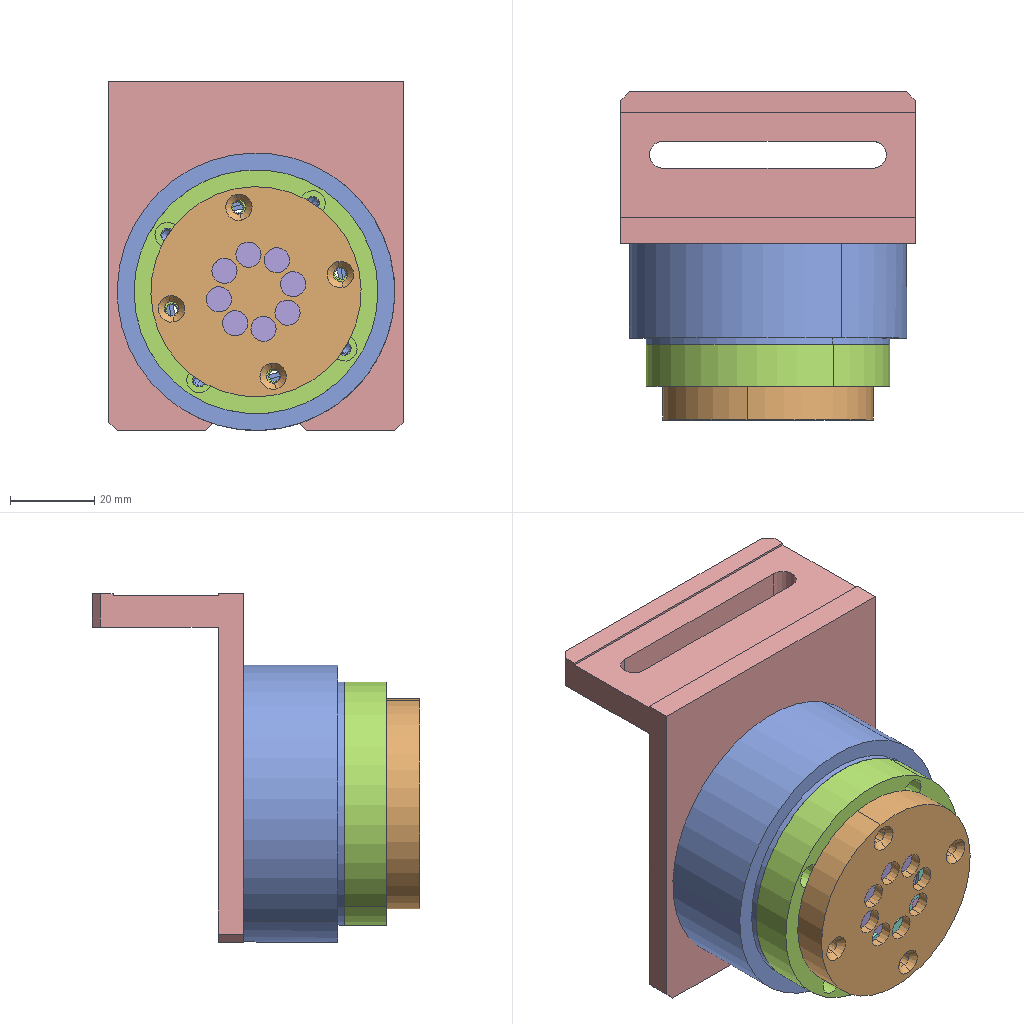Assembly | SolidWorks | 7 different items | 7 placed | box 70 x 78 x 83 mm
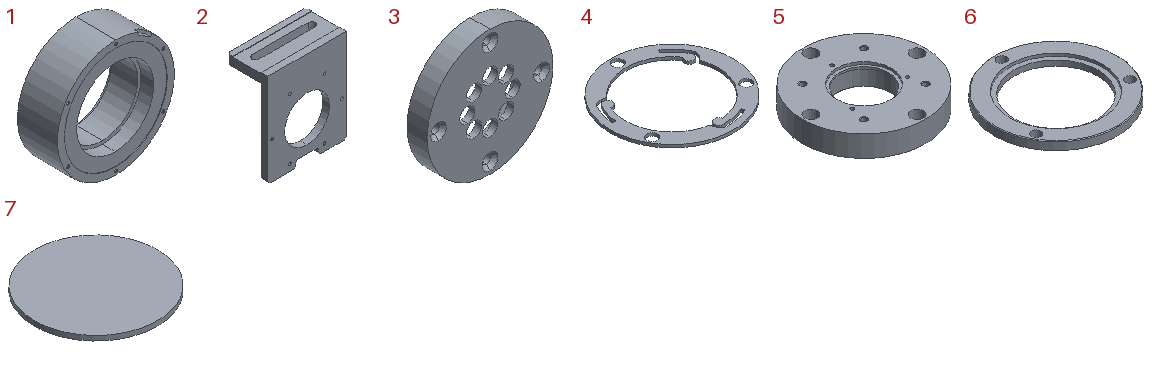Parts list (item | quantity | size | volume | features):
1 | x1 | 66 x 24 x 66 mm | 48084 mm3 | features ICE 7, HoleWzd 2, Extrusion 1
2 | x1 | 70 x 36 x 83 mm | 39637 mm3 | features ICE 6, Chamfer 1, Extrusion 1, Fillet 1
3 | x1 | 50 x 8 x 50 mm | 9503 mm3 | features ICE 2, Extrusion 1, HoleWzd 1
4 | x1 | 34 x 34 x 0.8 mm | 283.992 mm3 | features Fillet 3, ICE 3, CirPattern 2, DelFace 1, Extrusion 1
5 | x1 | 58 x 58 x 10 mm | 20570 mm3 | features ICE 7, Cut 2, HoleWzd 2, MoveFace 2, Chamfer 1, Extrusion 1
6 | x1 | 34 x 34 x 2.3 mm | 1004 mm3 | features ICE 6, Chamfer 2, Cut 2, HoleWzd 2, MoveFace 2, Extrusion 1
7 | x1 | 25.4 x 25.4 x 1 mm | 506.707 mm3 | features Extrusion 1
Mates (type | each side: item.copy, entity, surface, feature):
Concentric | 2.1 face cylinder Cut-Extrude1 | 1.1 face cylinder Boss-Extrude1
Coincident | 2.1 face plane Boss-Extrude1 | 1.1 face plane Boss-Extrude1
Concentric | 1.1 face cylinder Cut-Extrude1 | 5.1 face cylinder Boss-Extrude6
Coincident | 1.1 face plane Boss-Extrude2 | 5.1 face plane Boss-Extrude1
Concentric | 5.1 face cylinder Boss-Extrude1 | 6.1 face cylinder Boss-Extrude1
Coincident | 5.1 face plane Cut-Extrude3 | 6.1 face plane Boss-Extrude3
Concentric | 5.1 face cylinder Boss-Extrude1 | 4.1 face cylinder Cut-Extrude2
Coincident | 6.1 face plane Cut-Extrude3 | 4.1 face plane Boss-Extrude1
Concentric | 5.1 face cylinder Boss-Extrude6 | 3.1 face cylinder Boss-Extrude1
Coincident | 5.1 face plane Cut-Extrude3 | 3.1 face plane Boss-Extrude1
Concentric | 5.1 face cylinder Boss-Extrude1 | 7.1 face cylinder Boss-Extrude1
Coincident | 6.1 face plane Cut-Extrude4 | 7.1 face plane Boss-Extrude1